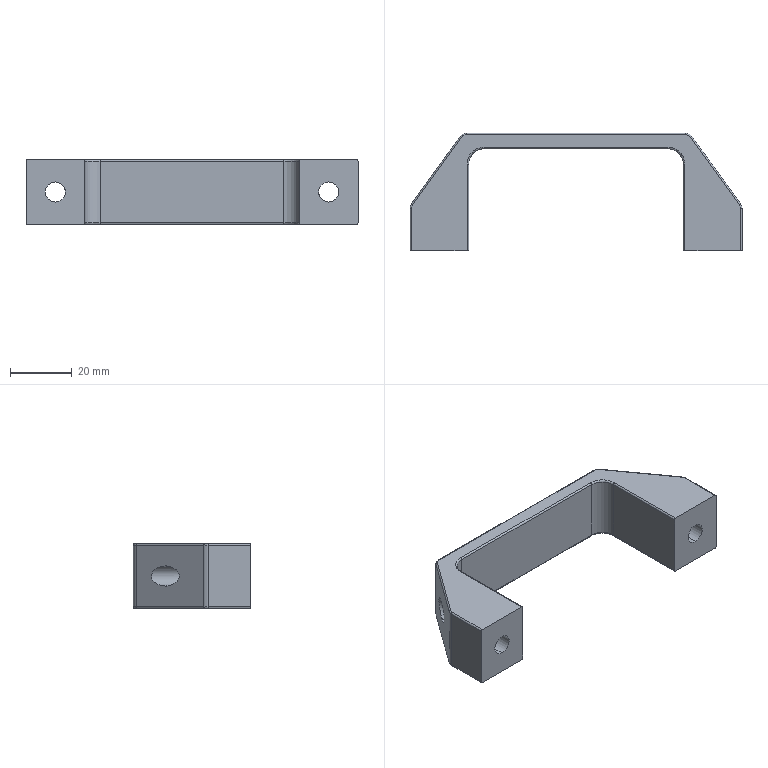Part | SolidWorks | features BaseBody 1 | 1 solid | 50 faces | box 107.5 x 38 x 21 mm | volume 27579 mm3 | cylinder 26 | plane 12 | spline 12 | commonest cylinder face diameters 1 x16 5 x4 6.5 x4 10 x2